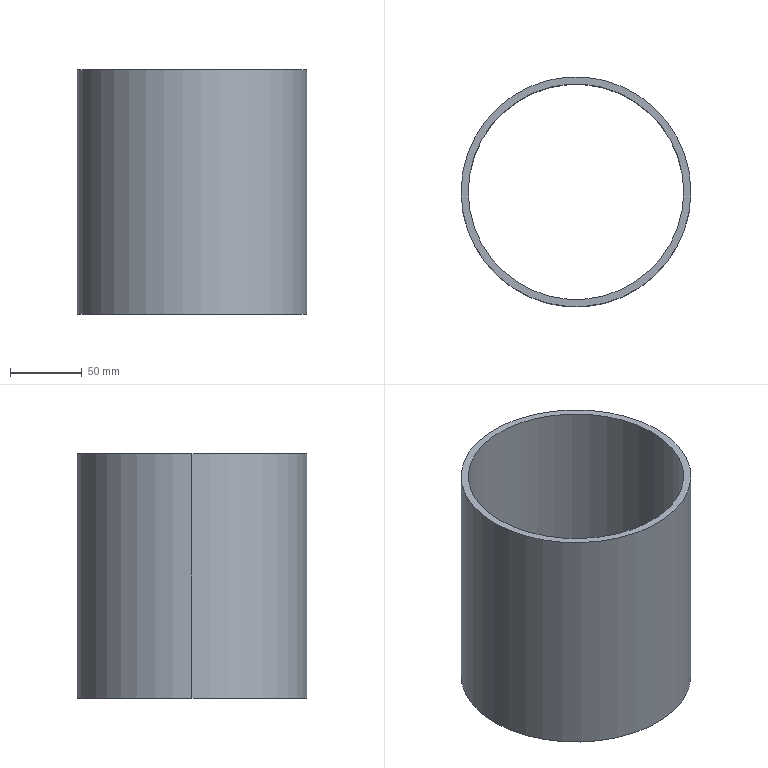Part | SolidWorks | features Extrusion 1 | 1 solid | 6 faces | box 160 x 160 x 170 mm | volume 413905 mm3 | cylinder 4 | plane 2 | commonest cylinder face diameters 150 x2 160 x2
STEP:
#1=CARTESIAN_POINT('',(-75.,0.,170.));
#2=VERTEX_POINT('',#1);
#3=CARTESIAN_POINT('',(75.,0.,170.));
#4=VERTEX_POINT('',#3);
#5=CARTESIAN_POINT('',(0.,0.,170.));
#6=DIRECTION('',(0.,0.,1.));
#7=DIRECTION('',(1.,0.,0.));
#8=AXIS2_PLACEMENT_3D('',#5,#6,#7);
#9=CIRCLE('',#8,75.);
#10=EDGE_CURVE('',#2,#4,#9,.T.);
#11=ORIENTED_EDGE('',*,*,#10,.T.);
#12=CARTESIAN_POINT('',(75.,0.,0.));
#13=VERTEX_POINT('',#12);
#14=CARTESIAN_POINT('',(75.,0.,170.));
#15=DIRECTION('',(0.,0.,-1.));
#16=VECTOR('',#15,1000.);
#17=LINE('',#14,#16);
#18=EDGE_CURVE('',#4,#13,#17,.T.);
#19=ORIENTED_EDGE('',*,*,#18,.T.);
#20=CARTESIAN_POINT('',(-75.,0.,0.));
#21=VERTEX_POINT('',#20);
#22=CARTESIAN_POINT('',(0.,0.,0.));
#23=DIRECTION('',(0.,0.,1.));
#24=DIRECTION('',(1.,0.,0.));
#25=AXIS2_PLACEMENT_3D('',#22,#23,#24);
#26=CIRCLE('',#25,75.);
#27=EDGE_CURVE('',#21,#13,#26,.T.);
#28=ORIENTED_EDGE('',*,*,#27,.F.);
#29=CARTESIAN_POINT('',(-75.,0.,170.));
#30=DIRECTION('',(0.,0.,-1.));
#31=VECTOR('',#30,1000.);
#32=LINE('',#29,#31);
#33=EDGE_CURVE('',#2,#21,#32,.T.);
#34=ORIENTED_EDGE('',*,*,#33,.F.);
#35=EDGE_LOOP('',(#11,#19,#28,#34));
#36=FACE_OUTER_BOUND('',#35,.T.);
#37=CARTESIAN_POINT('',(0.,0.,170.));
#38=DIRECTION('',(0.,0.,-1.));
#39=DIRECTION('',(-1.,0.,0.));
#40=AXIS2_PLACEMENT_3D('',#37,#38,#39);
#41=CYLINDRICAL_SURFACE('',#40,75.);
#42=ADVANCED_FACE('',(#36),#41,.F.);
#43=CARTESIAN_POINT('',(80.,0.,170.));
#44=VERTEX_POINT('',#43);
#45=CARTESIAN_POINT('',(-80.,0.,170.));
#46=VERTEX_POINT('',#45);
#47=CARTESIAN_POINT('',(0.,0.,170.));
#48=DIRECTION('',(0.,0.,1.));
#49=DIRECTION('',(1.,0.,0.));
#50=AXIS2_PLACEMENT_3D('',#47,#48,#49);
#51=CIRCLE('',#50,80.);
#52=EDGE_CURVE('',#44,#46,#51,.T.);
#53=ORIENTED_EDGE('',*,*,#52,.F.);
#54=CARTESIAN_POINT('',(80.,0.,0.));
#55=VERTEX_POINT('',#54);
#56=CARTESIAN_POINT('',(80.,0.,170.));
#57=DIRECTION('',(0.,0.,-1.));
#58=VECTOR('',#57,1000.);
#59=LINE('',#56,#58);
#60=EDGE_CURVE('',#44,#55,#59,.T.);
#61=ORIENTED_EDGE('',*,*,#60,.T.);
#62=CARTESIAN_POINT('',(-80.,0.,0.));
#63=VERTEX_POINT('',#62);
#64=CARTESIAN_POINT('',(0.,0.,0.));
#65=DIRECTION('',(0.,0.,1.));
#66=DIRECTION('',(1.,0.,0.));
#67=AXIS2_PLACEMENT_3D('',#64,#65,#66);
#68=CIRCLE('',#67,80.);
#69=EDGE_CURVE('',#55,#63,#68,.T.);
#70=ORIENTED_EDGE('',*,*,#69,.T.);
#71=CARTESIAN_POINT('',(-80.,0.,170.));
#72=DIRECTION('',(0.,0.,-1.));
#73=VECTOR('',#72,1000.);
#74=LINE('',#71,#73);
#75=EDGE_CURVE('',#46,#63,#74,.T.);
#76=ORIENTED_EDGE('',*,*,#75,.F.);
#77=EDGE_LOOP('',(#53,#61,#70,#76));
#78=FACE_OUTER_BOUND('',#77,.T.);
#79=CARTESIAN_POINT('',(0.,0.,170.));
#80=DIRECTION('',(0.,0.,-1.));
#81=DIRECTION('',(-1.,0.,0.));
#82=AXIS2_PLACEMENT_3D('',#79,#80,#81);
#83=CYLINDRICAL_SURFACE('',#82,80.);
#84=ADVANCED_FACE('',(#78),#83,.T.);
#85=CARTESIAN_POINT('',(0.,0.,170.));
#86=DIRECTION('',(0.,0.,1.));
#87=DIRECTION('',(1.,0.,0.));
#88=AXIS2_PLACEMENT_3D('',#85,#86,#87);
#89=CIRCLE('',#88,80.);
#90=EDGE_CURVE('',#46,#44,#89,.T.);
#91=ORIENTED_EDGE('',*,*,#90,.T.);
#92=ORIENTED_EDGE('',*,*,#52,.T.);
#93=EDGE_LOOP('',(#91,#92));
#94=FACE_OUTER_BOUND('',#93,.T.);
#95=ORIENTED_EDGE('',*,*,#10,.F.);
#96=CARTESIAN_POINT('',(0.,0.,170.));
#97=DIRECTION('',(0.,0.,1.));
#98=DIRECTION('',(1.,0.,0.));
#99=AXIS2_PLACEMENT_3D('',#96,#97,#98);
#100=CIRCLE('',#99,75.);
#101=EDGE_CURVE('',#4,#2,#100,.T.);
#102=ORIENTED_EDGE('',*,*,#101,.F.);
#103=EDGE_LOOP('',(#95,#102));
#104=FACE_BOUND('',#103,.T.);
#105=CARTESIAN_POINT('',(0.,0.,170.));
#106=DIRECTION('',(0.,0.,1.));
#107=DIRECTION('',(1.,0.,0.));
#108=AXIS2_PLACEMENT_3D('',#105,#106,#107);
#109=PLANE('',#108);
#110=ADVANCED_FACE('',(#94,#104),#109,.T.);
#111=CARTESIAN_POINT('',(0.,0.,0.));
#112=DIRECTION('',(0.,0.,1.));
#113=DIRECTION('',(1.,0.,0.));
#114=AXIS2_PLACEMENT_3D('',#111,#112,#113);
#115=CIRCLE('',#114,80.);
#116=EDGE_CURVE('',#63,#55,#115,.T.);
#117=ORIENTED_EDGE('',*,*,#116,.F.);
#118=ORIENTED_EDGE('',*,*,#69,.F.);
#119=EDGE_LOOP('',(#117,#118));
#120=FACE_OUTER_BOUND('',#119,.T.);
#121=ORIENTED_EDGE('',*,*,#27,.T.);
#122=CARTESIAN_POINT('',(0.,0.,0.));
#123=DIRECTION('',(0.,0.,1.));
#124=DIRECTION('',(1.,0.,0.));
#125=AXIS2_PLACEMENT_3D('',#122,#123,#124);
#126=CIRCLE('',#125,75.);
#127=EDGE_CURVE('',#13,#21,#126,.T.);
#128=ORIENTED_EDGE('',*,*,#127,.T.);
#129=EDGE_LOOP('',(#121,#128));
#130=FACE_BOUND('',#129,.T.);
#131=CARTESIAN_POINT('',(0.,0.,0.));
#132=DIRECTION('',(0.,0.,1.));
#133=DIRECTION('',(1.,0.,0.));
#134=AXIS2_PLACEMENT_3D('',#131,#132,#133);
#135=PLANE('',#134);
#136=ADVANCED_FACE('',(#120,#130),#135,.F.);
#137=ORIENTED_EDGE('',*,*,#60,.F.);
#138=ORIENTED_EDGE('',*,*,#90,.F.);
#139=ORIENTED_EDGE('',*,*,#75,.T.);
#140=ORIENTED_EDGE('',*,*,#116,.T.);
#141=EDGE_LOOP('',(#137,#138,#139,#140));
#142=FACE_OUTER_BOUND('',#141,.T.);
#143=CARTESIAN_POINT('',(0.,0.,170.));
#144=DIRECTION('',(0.,0.,-1.));
#145=DIRECTION('',(-1.,0.,0.));
#146=AXIS2_PLACEMENT_3D('',#143,#144,#145);
#147=CYLINDRICAL_SURFACE('',#146,80.);
#148=ADVANCED_FACE('',(#142),#147,.T.);
#149=ORIENTED_EDGE('',*,*,#18,.F.);
#150=ORIENTED_EDGE('',*,*,#101,.T.);
#151=ORIENTED_EDGE('',*,*,#33,.T.);
#152=ORIENTED_EDGE('',*,*,#127,.F.);
#153=EDGE_LOOP('',(#149,#150,#151,#152));
#154=FACE_OUTER_BOUND('',#153,.T.);
#155=CARTESIAN_POINT('',(0.,0.,170.));
#156=DIRECTION('',(0.,0.,-1.));
#157=DIRECTION('',(-1.,0.,0.));
#158=AXIS2_PLACEMENT_3D('',#155,#156,#157);
#159=CYLINDRICAL_SURFACE('',#158,75.);
#160=ADVANCED_FACE('',(#154),#159,.F.);
#161=CLOSED_SHELL('',(#42,#84,#110,#136,#148,#160));
#162=MANIFOLD_SOLID_BREP('',#161);
#163=CARTESIAN_POINT('',(0.,0.,0.));
#164=DIRECTION('',(0.,0.,1.));
#165=DIRECTION('',(1.,0.,0.));
#166=AXIS2_PLACEMENT_3D('',#163,#164,#165);
#167=(LENGTH_UNIT()NAMED_UNIT(*)SI_UNIT(.MILLI.,.METRE.));
#168=UNCERTAINTY_MEASURE_WITH_UNIT(LENGTH_MEASURE(0.00001),#167,'','');
#169=(NAMED_UNIT(*)PLANE_ANGLE_UNIT()SI_UNIT($,.RADIAN.));
#170=(NAMED_UNIT(*)SI_UNIT($,.STERADIAN.)SOLID_ANGLE_UNIT());
#171=(GEOMETRIC_REPRESENTATION_CONTEXT(3)GLOBAL_UNCERTAINTY_ASSIGNED_CONTEXT((#168))GLOBAL_UNIT_ASSIGNED_CONTEXT((#167,#169,#170))REPRESENTATION_CONTEXT('',''));
#172=ADVANCED_BREP_SHAPE_REPRESENTATION('',(#162,#166),#171);